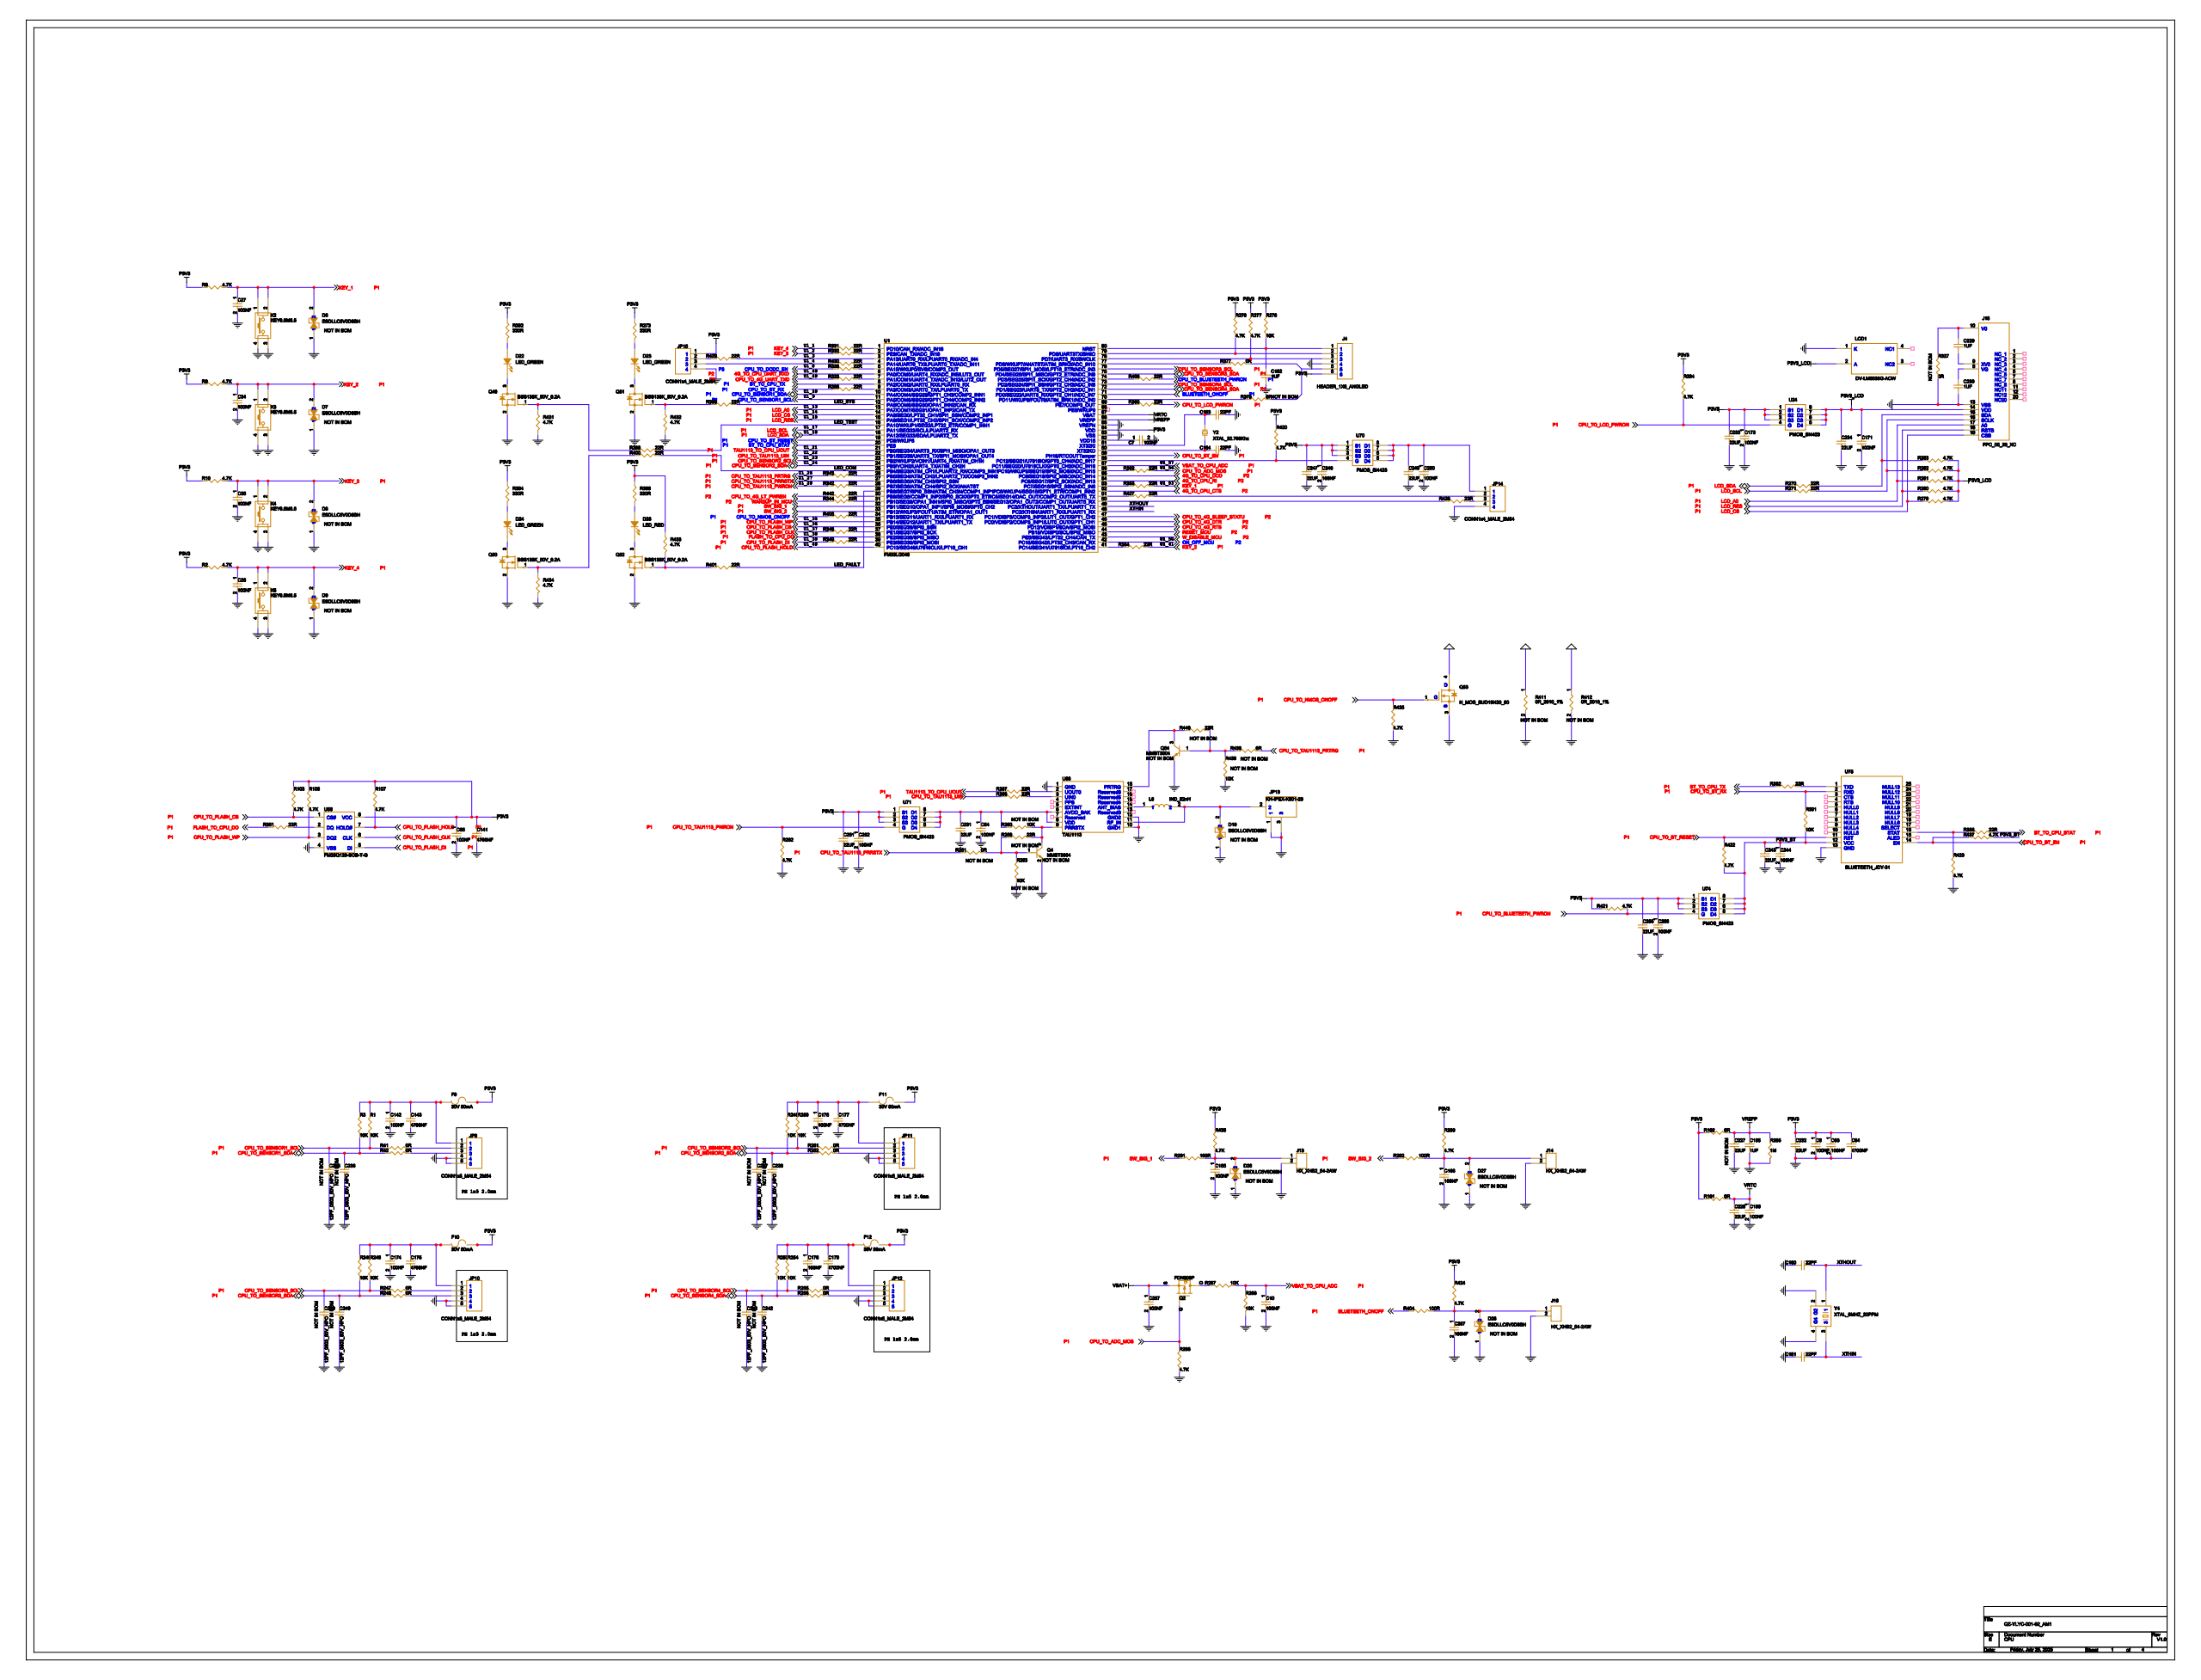Circuit board | Cadence Allegro | 366 parts | 230 nets | one sheet of the schematic
Parts on this sheet (reference | value | footprint):
C10 | C0603
C26 | C0603
C27 | C0603
C34 | C0603
C35 | C0603
C54 | C0603
C63 | C0603
C64 | C0603
C65 | C0603
C141 | C0603
C142 | C0603
C143 | C0603
C165 | C0603
C166 | C0603
C171 | C0603
C173 | C0603
C174 | C0603
C175 | C0603
C176 | C0603
C177 | C0603
C178 | C0603
C179 | C0603
C180 | C0603
C181 | C0603
C182 | C0603
C183 | C0603
C184 | C0603
C185 | C0603
C186 | C0603
C227 | C1206
C228 | C1206
C229 | C0603
C230 | C0603
C231 | C1206
C232 | C1206
C233 | C1206
C234 | C1206
C235 | C0603
C236 | C0603
C237 | C0603
C238 | C0603
C239 | C0603
C240 | C0603
C241 | C0603
C242 | C0603
C243 | C1206
C244 | C0603
C247 | C1206
C248 | C0603
C249 | C1206
C250 | C0603
C251 | C1206
C252 | C0603
C255 | C1206
C256 | C0603
C257 | C0603
C267 | C0603
D6 | DFN1006-2
D7 | DFN1006-2
D8 | DFN1006-2
D9 | DFN1006-2
D10 | DFN1006-2
D22 | LED1
D23 | LED1
D24 | LED1
D25 | LED1
D26 | DFN1006-2
D27 | DFN1006-2
D28 | DFN1006-2
F9 | 1210
F10 | 1210
F11 | 1210
F12 | 1210
J4 | HEADER_1X6_ANGLED
J13 | HX_XHB2_54-2AW
J14 | HX_XHB2_54-2AW
J15 | FPC_05_20_XC
J16 | HX_XHB2_54-2AW
JP9 | HX_XHB2_54-5AW
JP10 | HX_XHB2_54-5AW
JP11 | HX_XHB2_54-5AW
JP12 | HX_XHB2_54-5AW
JP13 | KH-IPEX-K501-29
JP14 | HX_XHB2_54-4AW
JP15 | HX_XHB2_54-4AW
K2 | ZX-QC66-65TP
K3 | ZX-QC66-65TP
K4 | ZX-QC66-65TP
K5 | ZX-QC66-65TP
L6 | IND_1008
LCD1 | LCD_70X43X6
Q2 | SOT_23_IRLML6402
Q4 | SOT23-123-095
Q49 | SOT23-123-095
Q50 | SOT23-123-095
Q51 | SOT23-123-095
Q52 | SOT23-123-095
Q53 | TO252-134
Q54 | SOT23-123-095
R1 | R0603
R2 | R0603
R3 | R0603
R8 | R0603
R9 | R0603
R10 | R0603
R41 | R0603
R42 | R0603
R101 | R1206
R102 | R1206
R103 | R0603
R106 | R0603
R107 | R0603
R245 | R0603
R246 | R0603
R247 | R0603
R248 | R0603
R249 | R0603
R250 | R0603
R251 | R0603
R252 | R0603
R253 | R0603
R254 | R0603
R255 | R0603
R256 | R0603
R257 | R0603
R258 | R0603
R259 | R0603
R260 | R0603
R261 | R0603
R262 | R0603
R263 | R0603
R270 | R0603
R271 | R0603
R273 | R0603
R276 | R0603
R277 | R0603
R278 | R0603
R279 | R0603
R280 | R0603
R281 | R0603
R282 | R0603
R283 | R0603
R284 | R0603
R285 | R0603
R286 | R0603
R287 | R0603
R288 | R0603
R290 | R0603
R291 | R0603
R292 | R0603
R327 | R1206
R331 | R0603
R332 | R0603
R333 | R0603
R338 | R0603
R342 | R0603
R343 | R0603
R344 | R0603
R348 | R0603
R349 | R0603
R351 | R0603
R352 | R0603
R353 | R0603
R354 | R0603
R360 | R0603
R377 | R0603
R378 | R0603
R382 | R0603
R385 | R0603
R386 | R0603
R388 | R0603
R391 | R0603
R392 | R0603
R394 | R0603
R398 | R0603
R399 | R0603
R400 | R0603
R401 | R0603
R404 | R0603
R406 | R0603
R409 | R0603
R411 | R2010
R412 | R2010
R420 | R0603
R421 | R0603
R422 | R0603
R423 | R0603
R424 | R0603
R427 | R0603
R428 | R0603
R429 | R0603
R430 | R0603
R431 | R0603
R432 | R0603
R433 | R0603
R434 | R0603
R435 | R0603
R436 | R0603
R437 | R0603
R438 | R0603
R439 | R0603
R440 | R0603
R442 | R0603
U1 | LQFP80
U24 | SO8
U56 | SOB_8_208MIL
U68 | TAU1113
U70 | SO8
U71 | SO8
U74 | SO8
U75 | BLUETEETH_JDY-31
Y2 | OSC_3215
Y4 | XTAL_5032_4P
Nets of these parts (net: part-pin ...):
GND_SIGNAL: Q53-4 R411-1 R412-1
VBAT+: C267-1 Q2-S
ON_OFF_MCU: U1-42
WAKEUP_IN_MCU: R344-1
RESET_MCU: U1-44
W_DISABLE_MCU: U1-43
GND: C10-2 C26-2 C27-2 C34-2 C35-2 C54-2 C63-2 C64-2 C65-2 C141-2 C142-2 C143-2 C165-2 C166-2 C171-2 C173-2 C174-2 C175-2 C176-2 C177-2 C178-2 C179-2 C180-1 C181-1 C182-2 C183-2 C184-2 C185-2 C186-2 C227-2 C228-2 C230-2 C231-2 C232-2 C233-2 C234-2 C235-2 C236-2 C237-2 C238-2 C239-2 C240-2 C241-2 C242-2 C243-2 C244-2 C247-2 C248-2 C249-2 C250-2 C251-2 C252-2 C255-2 C256-2 C257-2 C267-2 D6-1 D7-1 D8-1 D9-1 D10-1 D26-1 D27-1 D28-1 J4-4 J13-2 J14-2 J15-13 J16-2 JP9-4 JP9-5 JP10-4 JP10-5 JP11-4 JP11-5 JP12-4 JP12-5 JP13-1 JP13-3 JP14-4 JP15-4 K2-3 K2-4 K3-3 K3-4 K4-3 K4-4 K5-3 K5-4 LCD1-1 Q4-2 Q49-2 Q50-2 Q51-2 Q52-2 Q53-3 Q54-2 R262-1 R263-1 R285-2 R286-1 R288-2 R327-1 R411-2 R412-2 R423-1 R431-2 R432-2 R434-2 R435-1 R439-1 U56-4 U68-1 U68-10 U68-12 U75-13 Y4-2 Y4-4 U1-63 U1-65
CPU_TO_4G_UART_TXD: R333-1
XTHOUT: C180-2 Y4-1 U1-49
XTHIN: C181-2 Y4-3 U1-48
CPU_TO_BT_EN: R437-2 U75-14 U1-59
CPU_TO_BT_RESET: R422-2 U75-11 U1-19
CPU_TO_BT_RX: R386-1 R391-2 U75-2
N513713: R385-1 R423-2 U75-16
N512777: R382-2 U75-1
P3V3_BT: C243-1 C244-1 R391-1 R422-1 R437-1 U74-5 U74-6 U74-7 U74-8 U75-12
P3V3: C63-1 C64-1 C65-1 C141-1 C173-1 C232-1 C233-1 C247-1 C248-1 C251-1 C252-1 C255-1 C256-1 F9-1 F10-1 F11-1 F12-1 J4-6 JP15-1 R2-1 R8-1 R9-1 R10-1 R101-1 R102-1 R103-2 R106-2 R107-2 R273-1 R276-2 R277-2 R278-2 R284-2 R290-2 R388-1 R392-1 R394-1 R420-2 R421-2 R424-2 R433-1 R436-2 U24-1 U24-2 U24-3 U56-8 U70-1 U70-2 U70-3 U71-1 U71-2 U71-3 U74-1 U74-2 U74-3 U1-64
N154060: JP15-2 R429-1
U1_4: JP15-3 R430-1
N511239: C249-1 C250-1 JP14-1 U70-5 U70-6 U70-7 U70-8
N668731: JP14-2 R427-2
N668963: JP14-3 R428-2
N547255: D22-1 R392-2
N559067: D22-2 Q49-3
N559175: D23-1 R273-2
N559160: D23-2 Q51-3
N569796: D24-1 R394-2
N559115: D24-2 Q50-3
N530957: D25-1 R388-2
N569105: D25-2 Q52-3
N547317: Q49-1 R399-1 R431-1
N547869: Q50-1 R400-1 R434-1
N104537: Q51-1 R398-1 R432-1
N531041: Q52-1 R401-1 R433-2
CPU_TO_NMOS_ONOFF: Q53-1 R406-1 R435-2
N00255: D10-2 JP13-2 L6-2 U68-11
CPU_TO_DCDC_EN: R338-1
N00491: C184-1 Y2-1 U1-60
N00493: C183-1 Y2-2 U1-61
N583292: C257-1 D28-2 J16-1 R404-2 R424-1
VBAT_TO_CPU_ADC: C10-1 R287-1 R288-1 U1-57
N00347: C142-1 C143-1 F9-2 JP9-1 R1-2 R3-2
N206937: C165-1 D26-2 J13-1 R291-2 R436-1
N206816: C166-1 D27-2 J14-1 R290-1 R292-2
P3V3_LCD: C171-1 C234-1 J15-14 LCD1-2 R279-1 R280-1 R281-1 R282-1 R283-1 U24-5 U24-6 U24-7 U24-8
N204409: C174-1 C175-1 F10-2 JP10-1 R245-2 R246-2
N00397: C176-1 C177-1 F11-2 JP11-1 R249-2 R250-2
N205183: C178-1 C179-1 F12-2 JP12-1 R253-2 R254-2
VRTC: C186-1 C228-1 R101-2 U1-67
KEY_4: C26-1 D9-2 K5-1 K5-2 R2-2 R331-1
KEY_1: C27-1 D6-2 K2-1 K2-2 R8-2 R353-2
KEY_2: C34-1 D7-2 K3-1 K3-2 R9-2 R354-2
KEY_3: C35-1 D8-2 K4-1 K4-2 R10-2 R332-1
N00283: C54-1 C231-1 R260-1 U68-6 U68-8 U71-5 U71-6 U71-7 U71-8
VREFP: C185-1 C227-1 R102-2 R285-1 U1-66
N00233: C182-1 J4-1 R278-1 U1-80
N415475: C229-1 J15-10 R327-2
N415482: C229-2 J15-9
N415489: C230-1 J15-6
CPU_TO_SENSOR1_SCL: C235-1 R1-1 R41-1 U1-11
CPU_TO_SENSOR1_SDA: C236-1 R3-1 R42-1 U1-10
CPU_TO_SENSOR2_SCL: C237-1 R250-1 R251-1 U1-23
CPU_TO_SENSOR2_SDA: C238-1 R249-1 R252-1 U1-24
CPU_TO_SENSOR3_SCL: C239-1 R246-1 R247-1 U1-76
CPU_TO_SENSOR3_SDA: C240-1 R245-1 R248-1 U1-75
CPU_TO_SENSOR4_SCL: C241-1 R254-1 R255-1 U1-73
CPU_TO_SENSOR4_SDA: C242-1 R253-1 R256-1 U1-72
LCD_A0: J15-17 R281-2 U1-13
LCD_CS: J15-19 R279-2 U1-14
LCD_RES: J15-18 R280-2 U1-15
N189974: J15-16 R271-2 R282-2
N189937: J15-15 R270-2 R283-2
N00237: J4-2 R276-1 U1-79
N00239: J4-3 R277-1 U1-78
N00243: J4-5 R377-2 R378-2
N204665: JP10-2 R247-2
N204679: JP10-3 R248-2
N00403: JP11-2 R251-2
N00411: JP11-3 R252-2
N205443: JP12-2 R255-2
N205457: JP12-3 R256-2
N00353: JP9-2 R41-2
N00361: JP9-3 R42-2
N00253: L6-1 U68-14
CPU_TO_4G_LT_PWREN: R442-1
N160557: Q2-D R287-2
CPU_TO_ADC_MOS: Q2-G R286-2 R352-2
N721396: Q54-1 R438-1 R439-2 R440-2
N720292: Q54-3 R440-1 U68-18
CPU_TO_4G_SLEEP_STATU: U1-47
CPU_TO_4G_DTR: U1-46
CPU_TO_4G_RTS: U1-45
4G_TO_CPU_DCD: U1-55
4G_TO_CPU_RI: U1-54
4G_TO_CPU_CTS: U1-52
N175668: Q4-1 R259-1 R261-2 R263-2
N00297: Q4-3 R259-2 R260-2 U68-9
CPU_TO_TAU1113_PRTRG: R343-1 R438-2
CPU_TO_TAU1113_PRRSTX: R261-1 U1-27
N00241: R377-1 U1-77
N443471: R378-1 U1-70
N744145: R442-2 U1-30
N511267: R427-1 U1-51
N511273: R428-1 U1-50
U1_3: R429-2 U1-3
N669053: R430-2 U1-4
BT_TO_CPU_TX: R382-1 U1-8
BT_TO_CPU_STAT: R385-2 U1-20
N521081: R386-2 U1-9
LED_SYS: R398-2 U1-12
LED_TEST: R399-2 U1-16
LED_COM: R400-2 U1-25
LED_FAULT: R401-2 U1-29
N612607: R406-2 U1-34
N583078: R409-1 U1-74
CPU_TO_BLUETEETH_PWRON: R409-2 R421-1 U74-4
N436105: R331-2 U1-1
N436173: R332-2 U1-2
N436259: R333-2 U1-7
4G_TO_CPU_UART_RXD: U1-6
N520933: R338-2 U1-5
CPU_TO_TAU1113_PWRON: R262-2 R342-1 U71-4
N436783: R342-2 U1-28
N436835: R343-2 U1-26
N436885: R344-2 U1-31
CPU_TO_FLASH_CLK: R348-1 U56-6
N437149: R348-2 U1-37
CPU_TO_FLASH_DI: R349-1 U56-5
N437195: R349-2 U1-39
FLASH_TO_CPU_DO: R351-1 U1-38
N437365: R351-2 U56-2
N00519: R352-1 U1-56
N00515: R353-1 U1-53
N00503: R354-1 U1-41
N180604: R360-1 U1-69
CPU_TO_LCD_PWRON: R284-1 R360-2 U24-4
TAU1113_TO_CPU_UOUT: R257-1 U1-21
N00271: R257-2 U68-2
CPU_TO_TAU1113_UIN: R258-1 U1-22
N00273: R258-2 U68-3
LCD_SDA: R270-1 U1-18
LCD_SCL: R271-1 U1-17
BLUETEETH_ONOFF: R404-1 U1-71
SW_SIG_1: R291-1 U1-32
SW_SIG_2: R292-1 U1-33
CPU_TO_FLASH_CS: R103-1 U56-1 U1-36
CPU_TO_FLASH_WP: R106-1 U56-3 U1-35
CPU_TO_FLASH_HOLD: R107-1 U56-7 U1-40
N521527: R420-1 U70-4 U1-58